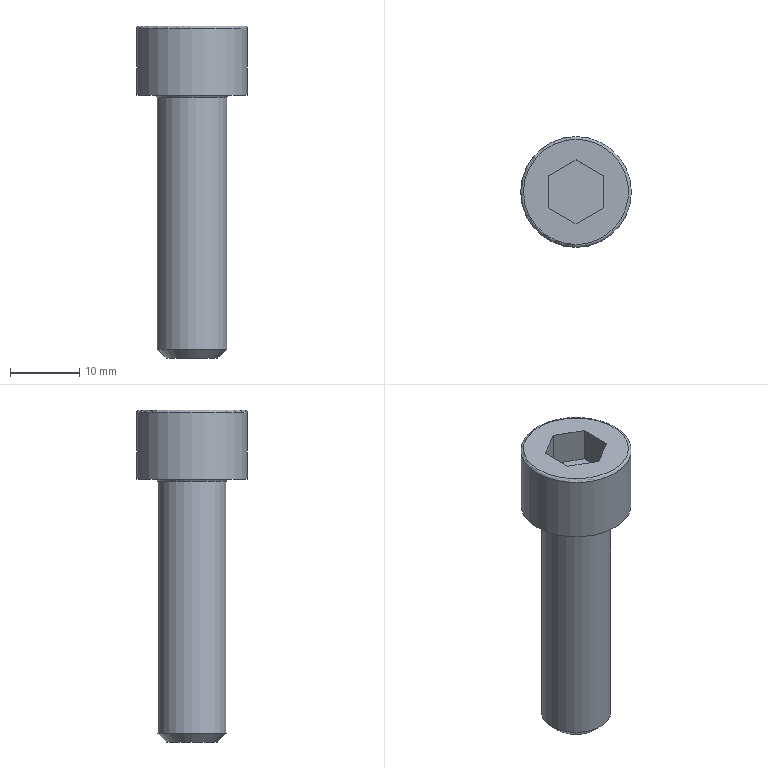Part | STEP file | solid 165 | 1 solid | 15 faces | box 16 x 16 x 48 mm | volume 4695 mm3 | plane 10 | cylinder 2 | torus 2 | cone 1 | commonest cylinder face diameters 10 x1 16 x1